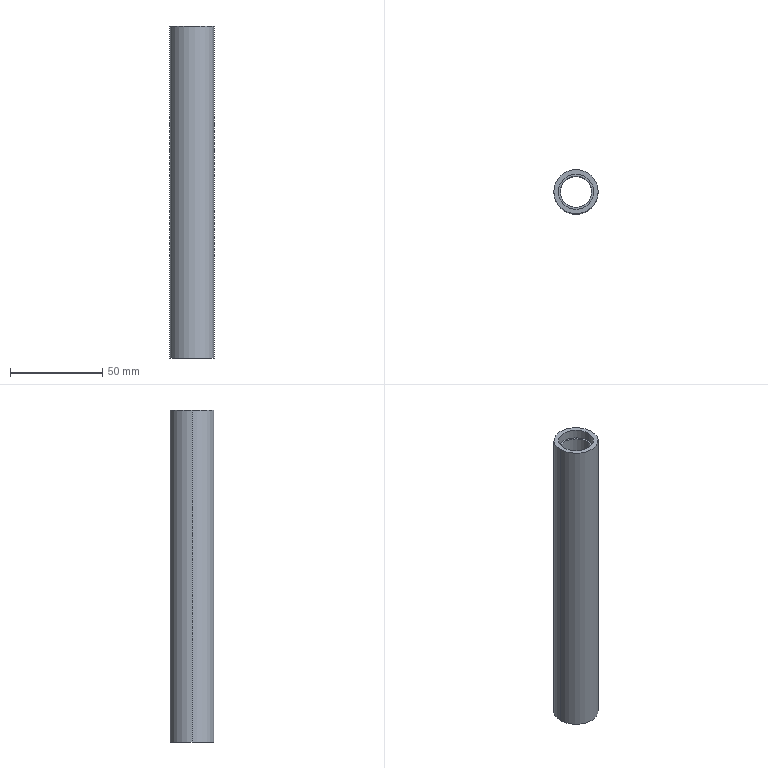Part | STEP file | MT-COMBO-119-S034 | 1 solid | 12 faces | box 24 x 24 x 180 mm | volume 40008 mm3 | cylinder 8 | plane 4 | commonest cylinder face diameters 19 x4 17 x2 24 x2
STEP:
#1=CARTESIAN_POINT('',(9.5,0.,5.));
#2=VERTEX_POINT('',#1);
#3=CARTESIAN_POINT('',(-9.5,0.,5.));
#4=VERTEX_POINT('',#3);
#5=CARTESIAN_POINT('',(0.,0.,5.));
#6=DIRECTION('',(0.,0.,-1.));
#7=DIRECTION('',(-1.,0.,0.));
#8=AXIS2_PLACEMENT_3D('',#5,#6,#7);
#9=CIRCLE('',#8,9.5);
#10=EDGE_CURVE('',#2,#4,#9,.T.);
#11=ORIENTED_EDGE('',*,*,#10,.F.);
#12=CARTESIAN_POINT('',(9.5,0.,0.));
#13=VERTEX_POINT('',#12);
#14=CARTESIAN_POINT('',(9.5,0.,5.));
#15=DIRECTION('',(0.,0.,-1.));
#16=VECTOR('',#15,1000.);
#17=LINE('',#14,#16);
#18=EDGE_CURVE('',#2,#13,#17,.T.);
#19=ORIENTED_EDGE('',*,*,#18,.T.);
#20=CARTESIAN_POINT('',(-9.5,0.,0.));
#21=VERTEX_POINT('',#20);
#22=CARTESIAN_POINT('',(0.,0.,0.));
#23=DIRECTION('',(0.,0.,-1.));
#24=DIRECTION('',(-1.,0.,0.));
#25=AXIS2_PLACEMENT_3D('',#22,#23,#24);
#26=CIRCLE('',#25,9.5);
#27=EDGE_CURVE('',#13,#21,#26,.T.);
#28=ORIENTED_EDGE('',*,*,#27,.T.);
#29=CARTESIAN_POINT('',(-9.5,0.,5.));
#30=DIRECTION('',(0.,0.,-1.));
#31=VECTOR('',#30,1000.);
#32=LINE('',#29,#31);
#33=EDGE_CURVE('',#4,#21,#32,.T.);
#34=ORIENTED_EDGE('',*,*,#33,.F.);
#35=EDGE_LOOP('',(#11,#19,#28,#34));
#36=FACE_OUTER_BOUND('',#35,.T.);
#37=CARTESIAN_POINT('',(0.,0.,5.));
#38=DIRECTION('',(0.,0.,-1.));
#39=DIRECTION('',(-1.,0.,0.));
#40=AXIS2_PLACEMENT_3D('',#37,#38,#39);
#41=CYLINDRICAL_SURFACE('',#40,9.5);
#42=ADVANCED_FACE('',(#36),#41,.F.);
#43=CARTESIAN_POINT('',(-9.5,0.,175.));
#44=VERTEX_POINT('',#43);
#45=CARTESIAN_POINT('',(9.5,0.,175.));
#46=VERTEX_POINT('',#45);
#47=CARTESIAN_POINT('',(0.,0.,175.));
#48=DIRECTION('',(0.,0.,1.));
#49=DIRECTION('',(1.,0.,0.));
#50=AXIS2_PLACEMENT_3D('',#47,#48,#49);
#51=CIRCLE('',#50,9.5);
#52=EDGE_CURVE('',#44,#46,#51,.T.);
#53=ORIENTED_EDGE('',*,*,#52,.F.);
#54=CARTESIAN_POINT('',(-9.5,0.,180.));
#55=VERTEX_POINT('',#54);
#56=CARTESIAN_POINT('',(-9.5,0.,175.));
#57=DIRECTION('',(0.,0.,1.));
#58=VECTOR('',#57,1000.);
#59=LINE('',#56,#58);
#60=EDGE_CURVE('',#44,#55,#59,.T.);
#61=ORIENTED_EDGE('',*,*,#60,.T.);
#62=CARTESIAN_POINT('',(9.5,0.,180.));
#63=VERTEX_POINT('',#62);
#64=CARTESIAN_POINT('',(0.,0.,180.));
#65=DIRECTION('',(0.,0.,1.));
#66=DIRECTION('',(1.,0.,0.));
#67=AXIS2_PLACEMENT_3D('',#64,#65,#66);
#68=CIRCLE('',#67,9.5);
#69=EDGE_CURVE('',#55,#63,#68,.T.);
#70=ORIENTED_EDGE('',*,*,#69,.T.);
#71=CARTESIAN_POINT('',(9.5,0.,175.));
#72=DIRECTION('',(0.,0.,1.));
#73=VECTOR('',#72,1000.);
#74=LINE('',#71,#73);
#75=EDGE_CURVE('',#46,#63,#74,.T.);
#76=ORIENTED_EDGE('',*,*,#75,.F.);
#77=EDGE_LOOP('',(#53,#61,#70,#76));
#78=FACE_OUTER_BOUND('',#77,.T.);
#79=CARTESIAN_POINT('',(0.,0.,175.));
#80=DIRECTION('',(0.,0.,1.));
#81=DIRECTION('',(1.,0.,0.));
#82=AXIS2_PLACEMENT_3D('',#79,#80,#81);
#83=CYLINDRICAL_SURFACE('',#82,9.5);
#84=ADVANCED_FACE('',(#78),#83,.F.);
#85=CARTESIAN_POINT('',(12.,0.,180.));
#86=VERTEX_POINT('',#85);
#87=CARTESIAN_POINT('',(-12.,0.,180.));
#88=VERTEX_POINT('',#87);
#89=CARTESIAN_POINT('',(0.,0.,180.));
#90=DIRECTION('',(0.,0.,1.));
#91=DIRECTION('',(1.,0.,0.));
#92=AXIS2_PLACEMENT_3D('',#89,#90,#91);
#93=CIRCLE('',#92,12.);
#94=EDGE_CURVE('',#86,#88,#93,.T.);
#95=ORIENTED_EDGE('',*,*,#94,.F.);
#96=CARTESIAN_POINT('',(12.,0.,0.));
#97=VERTEX_POINT('',#96);
#98=CARTESIAN_POINT('',(12.,0.,180.));
#99=DIRECTION('',(0.,0.,-1.));
#100=VECTOR('',#99,1000.);
#101=LINE('',#98,#100);
#102=EDGE_CURVE('',#86,#97,#101,.T.);
#103=ORIENTED_EDGE('',*,*,#102,.T.);
#104=CARTESIAN_POINT('',(-12.,0.,0.));
#105=VERTEX_POINT('',#104);
#106=CARTESIAN_POINT('',(0.,0.,0.));
#107=DIRECTION('',(0.,0.,1.));
#108=DIRECTION('',(1.,0.,0.));
#109=AXIS2_PLACEMENT_3D('',#106,#107,#108);
#110=CIRCLE('',#109,12.);
#111=EDGE_CURVE('',#97,#105,#110,.T.);
#112=ORIENTED_EDGE('',*,*,#111,.T.);
#113=CARTESIAN_POINT('',(-12.,0.,180.));
#114=DIRECTION('',(0.,0.,-1.));
#115=VECTOR('',#114,1000.);
#116=LINE('',#113,#115);
#117=EDGE_CURVE('',#88,#105,#116,.T.);
#118=ORIENTED_EDGE('',*,*,#117,.F.);
#119=EDGE_LOOP('',(#95,#103,#112,#118));
#120=FACE_OUTER_BOUND('',#119,.T.);
#121=CARTESIAN_POINT('',(0.,0.,180.));
#122=DIRECTION('',(0.,0.,-1.));
#123=DIRECTION('',(-1.,0.,0.));
#124=AXIS2_PLACEMENT_3D('',#121,#122,#123);
#125=CYLINDRICAL_SURFACE('',#124,12.);
#126=ADVANCED_FACE('',(#120),#125,.T.);
#127=CARTESIAN_POINT('',(-8.5,0.,5.));
#128=VERTEX_POINT('',#127);
#129=CARTESIAN_POINT('',(8.5,0.,5.));
#130=VERTEX_POINT('',#129);
#131=CARTESIAN_POINT('',(0.,0.,5.));
#132=DIRECTION('',(0.,0.,1.));
#133=DIRECTION('',(-1.,0.,0.));
#134=AXIS2_PLACEMENT_3D('',#131,#132,#133);
#135=CIRCLE('',#134,8.5);
#136=EDGE_CURVE('',#128,#130,#135,.T.);
#137=ORIENTED_EDGE('',*,*,#136,.F.);
#138=CARTESIAN_POINT('',(-8.5,0.,175.));
#139=VERTEX_POINT('',#138);
#140=CARTESIAN_POINT('',(-8.5,0.,0.));
#141=DIRECTION('',(0.,0.,1.));
#142=VECTOR('',#141,1000.);
#143=LINE('',#140,#142);
#144=EDGE_CURVE('',#128,#139,#143,.T.);
#145=ORIENTED_EDGE('',*,*,#144,.T.);
#146=CARTESIAN_POINT('',(8.5,0.,175.));
#147=VERTEX_POINT('',#146);
#148=CARTESIAN_POINT('',(0.,0.,175.));
#149=DIRECTION('',(0.,0.,1.));
#150=DIRECTION('',(1.,0.,0.));
#151=AXIS2_PLACEMENT_3D('',#148,#149,#150);
#152=CIRCLE('',#151,8.5);
#153=EDGE_CURVE('',#139,#147,#152,.T.);
#154=ORIENTED_EDGE('',*,*,#153,.T.);
#155=CARTESIAN_POINT('',(8.5,0.,0.));
#156=DIRECTION('',(0.,0.,1.));
#157=VECTOR('',#156,1000.);
#158=LINE('',#155,#157);
#159=EDGE_CURVE('',#130,#147,#158,.T.);
#160=ORIENTED_EDGE('',*,*,#159,.F.);
#161=EDGE_LOOP('',(#137,#145,#154,#160));
#162=FACE_OUTER_BOUND('',#161,.T.);
#163=CARTESIAN_POINT('',(0.,0.,0.));
#164=DIRECTION('',(0.,0.,1.));
#165=DIRECTION('',(1.,0.,0.));
#166=AXIS2_PLACEMENT_3D('',#163,#164,#165);
#167=CYLINDRICAL_SURFACE('',#166,8.5);
#168=ADVANCED_FACE('',(#162),#167,.F.);
#169=ORIENTED_EDGE('',*,*,#144,.F.);
#170=CARTESIAN_POINT('',(0.,0.,5.));
#171=DIRECTION('',(0.,0.,1.));
#172=DIRECTION('',(-1.,0.,0.));
#173=AXIS2_PLACEMENT_3D('',#170,#171,#172);
#174=CIRCLE('',#173,8.5);
#175=EDGE_CURVE('',#130,#128,#174,.T.);
#176=ORIENTED_EDGE('',*,*,#175,.F.);
#177=ORIENTED_EDGE('',*,*,#159,.T.);
#178=CARTESIAN_POINT('',(0.,0.,175.));
#179=DIRECTION('',(0.,0.,1.));
#180=DIRECTION('',(1.,0.,0.));
#181=AXIS2_PLACEMENT_3D('',#178,#179,#180);
#182=CIRCLE('',#181,8.5);
#183=EDGE_CURVE('',#147,#139,#182,.T.);
#184=ORIENTED_EDGE('',*,*,#183,.T.);
#185=EDGE_LOOP('',(#169,#176,#177,#184));
#186=FACE_OUTER_BOUND('',#185,.T.);
#187=CARTESIAN_POINT('',(0.,0.,0.));
#188=DIRECTION('',(0.,0.,1.));
#189=DIRECTION('',(1.,0.,0.));
#190=AXIS2_PLACEMENT_3D('',#187,#188,#189);
#191=CYLINDRICAL_SURFACE('',#190,8.5);
#192=ADVANCED_FACE('',(#186),#191,.F.);
#193=ORIENTED_EDGE('',*,*,#102,.F.);
#194=CARTESIAN_POINT('',(0.,0.,180.));
#195=DIRECTION('',(0.,0.,1.));
#196=DIRECTION('',(1.,0.,0.));
#197=AXIS2_PLACEMENT_3D('',#194,#195,#196);
#198=CIRCLE('',#197,12.);
#199=EDGE_CURVE('',#88,#86,#198,.T.);
#200=ORIENTED_EDGE('',*,*,#199,.F.);
#201=ORIENTED_EDGE('',*,*,#117,.T.);
#202=CARTESIAN_POINT('',(0.,0.,0.));
#203=DIRECTION('',(0.,0.,1.));
#204=DIRECTION('',(1.,0.,0.));
#205=AXIS2_PLACEMENT_3D('',#202,#203,#204);
#206=CIRCLE('',#205,12.);
#207=EDGE_CURVE('',#105,#97,#206,.T.);
#208=ORIENTED_EDGE('',*,*,#207,.T.);
#209=EDGE_LOOP('',(#193,#200,#201,#208));
#210=FACE_OUTER_BOUND('',#209,.T.);
#211=CARTESIAN_POINT('',(0.,0.,180.));
#212=DIRECTION('',(0.,0.,-1.));
#213=DIRECTION('',(-1.,0.,0.));
#214=AXIS2_PLACEMENT_3D('',#211,#212,#213);
#215=CYLINDRICAL_SURFACE('',#214,12.);
#216=ADVANCED_FACE('',(#210),#215,.T.);
#217=CARTESIAN_POINT('',(0.,0.,180.));
#218=DIRECTION('',(0.,0.,1.));
#219=DIRECTION('',(1.,0.,0.));
#220=AXIS2_PLACEMENT_3D('',#217,#218,#219);
#221=CIRCLE('',#220,9.5);
#222=EDGE_CURVE('',#63,#55,#221,.T.);
#223=ORIENTED_EDGE('',*,*,#222,.F.);
#224=ORIENTED_EDGE('',*,*,#69,.F.);
#225=EDGE_LOOP('',(#223,#224));
#226=FACE_BOUND('',#225,.T.);
#227=ORIENTED_EDGE('',*,*,#199,.T.);
#228=ORIENTED_EDGE('',*,*,#94,.T.);
#229=EDGE_LOOP('',(#227,#228));
#230=FACE_OUTER_BOUND('',#229,.T.);
#231=CARTESIAN_POINT('',(0.,0.,180.));
#232=DIRECTION('',(0.,0.,1.));
#233=DIRECTION('',(1.,0.,0.));
#234=AXIS2_PLACEMENT_3D('',#231,#232,#233);
#235=PLANE('',#234);
#236=ADVANCED_FACE('',(#226,#230),#235,.T.);
#237=CARTESIAN_POINT('',(0.,0.,0.));
#238=DIRECTION('',(0.,0.,-1.));
#239=DIRECTION('',(-1.,0.,0.));
#240=AXIS2_PLACEMENT_3D('',#237,#238,#239);
#241=CIRCLE('',#240,9.5);
#242=EDGE_CURVE('',#21,#13,#241,.T.);
#243=ORIENTED_EDGE('',*,*,#242,.F.);
#244=ORIENTED_EDGE('',*,*,#27,.F.);
#245=EDGE_LOOP('',(#243,#244));
#246=FACE_BOUND('',#245,.T.);
#247=ORIENTED_EDGE('',*,*,#207,.F.);
#248=ORIENTED_EDGE('',*,*,#111,.F.);
#249=EDGE_LOOP('',(#247,#248));
#250=FACE_OUTER_BOUND('',#249,.T.);
#251=CARTESIAN_POINT('',(0.,0.,0.));
#252=DIRECTION('',(0.,0.,1.));
#253=DIRECTION('',(1.,0.,0.));
#254=AXIS2_PLACEMENT_3D('',#251,#252,#253);
#255=PLANE('',#254);
#256=ADVANCED_FACE('',(#246,#250),#255,.F.);
#257=ORIENTED_EDGE('',*,*,#60,.F.);
#258=CARTESIAN_POINT('',(0.,0.,175.));
#259=DIRECTION('',(0.,0.,1.));
#260=DIRECTION('',(1.,0.,0.));
#261=AXIS2_PLACEMENT_3D('',#258,#259,#260);
#262=CIRCLE('',#261,9.5);
#263=EDGE_CURVE('',#46,#44,#262,.T.);
#264=ORIENTED_EDGE('',*,*,#263,.F.);
#265=ORIENTED_EDGE('',*,*,#75,.T.);
#266=ORIENTED_EDGE('',*,*,#222,.T.);
#267=EDGE_LOOP('',(#257,#264,#265,#266));
#268=FACE_OUTER_BOUND('',#267,.T.);
#269=CARTESIAN_POINT('',(0.,0.,175.));
#270=DIRECTION('',(0.,0.,1.));
#271=DIRECTION('',(1.,0.,0.));
#272=AXIS2_PLACEMENT_3D('',#269,#270,#271);
#273=CYLINDRICAL_SURFACE('',#272,9.5);
#274=ADVANCED_FACE('',(#268),#273,.F.);
#275=ORIENTED_EDGE('',*,*,#183,.F.);
#276=ORIENTED_EDGE('',*,*,#153,.F.);
#277=EDGE_LOOP('',(#275,#276));
#278=FACE_BOUND('',#277,.T.);
#279=ORIENTED_EDGE('',*,*,#263,.T.);
#280=ORIENTED_EDGE('',*,*,#52,.T.);
#281=EDGE_LOOP('',(#279,#280));
#282=FACE_OUTER_BOUND('',#281,.T.);
#283=CARTESIAN_POINT('',(0.,0.,175.));
#284=DIRECTION('',(0.,0.,1.));
#285=DIRECTION('',(1.,0.,0.));
#286=AXIS2_PLACEMENT_3D('',#283,#284,#285);
#287=PLANE('',#286);
#288=ADVANCED_FACE('',(#278,#282),#287,.T.);
#289=CARTESIAN_POINT('',(0.,0.,5.));
#290=DIRECTION('',(0.,0.,-1.));
#291=DIRECTION('',(-1.,0.,0.));
#292=AXIS2_PLACEMENT_3D('',#289,#290,#291);
#293=CIRCLE('',#292,9.5);
#294=EDGE_CURVE('',#4,#2,#293,.T.);
#295=ORIENTED_EDGE('',*,*,#294,.T.);
#296=ORIENTED_EDGE('',*,*,#10,.T.);
#297=EDGE_LOOP('',(#295,#296));
#298=FACE_OUTER_BOUND('',#297,.T.);
#299=ORIENTED_EDGE('',*,*,#175,.T.);
#300=ORIENTED_EDGE('',*,*,#136,.T.);
#301=EDGE_LOOP('',(#299,#300));
#302=FACE_BOUND('',#301,.T.);
#303=CARTESIAN_POINT('',(0.,0.,5.));
#304=DIRECTION('',(0.,0.,-1.));
#305=DIRECTION('',(-1.,0.,0.));
#306=AXIS2_PLACEMENT_3D('',#303,#304,#305);
#307=PLANE('',#306);
#308=ADVANCED_FACE('',(#298,#302),#307,.T.);
#309=ORIENTED_EDGE('',*,*,#18,.F.);
#310=ORIENTED_EDGE('',*,*,#294,.F.);
#311=ORIENTED_EDGE('',*,*,#33,.T.);
#312=ORIENTED_EDGE('',*,*,#242,.T.);
#313=EDGE_LOOP('',(#309,#310,#311,#312));
#314=FACE_OUTER_BOUND('',#313,.T.);
#315=CARTESIAN_POINT('',(0.,0.,5.));
#316=DIRECTION('',(0.,0.,-1.));
#317=DIRECTION('',(-1.,0.,0.));
#318=AXIS2_PLACEMENT_3D('',#315,#316,#317);
#319=CYLINDRICAL_SURFACE('',#318,9.5);
#320=ADVANCED_FACE('',(#314),#319,.F.);
#321=CLOSED_SHELL('',(#42,#84,#126,#168,#192,#216,#236,#256,#274,#288,#308,#320));
#322=MANIFOLD_SOLID_BREP('',#321);
#323=CARTESIAN_POINT('',(0.,0.,0.));
#324=DIRECTION('',(0.,0.,1.));
#325=DIRECTION('',(1.,0.,0.));
#326=AXIS2_PLACEMENT_3D('',#323,#324,#325);
#327=(LENGTH_UNIT()NAMED_UNIT(*)SI_UNIT(.MILLI.,.METRE.));
#328=UNCERTAINTY_MEASURE_WITH_UNIT(LENGTH_MEASURE(0.00001),#327,'','');
#329=(NAMED_UNIT(*)PLANE_ANGLE_UNIT()SI_UNIT($,.RADIAN.));
#330=(NAMED_UNIT(*)SI_UNIT($,.STERADIAN.)SOLID_ANGLE_UNIT());
#331=(GEOMETRIC_REPRESENTATION_CONTEXT(3)GLOBAL_UNCERTAINTY_ASSIGNED_CONTEXT((#328))GLOBAL_UNIT_ASSIGNED_CONTEXT((#327,#329,#330))REPRESENTATION_CONTEXT('',''));
#332=ADVANCED_BREP_SHAPE_REPRESENTATION('',(#322,#326),#331);